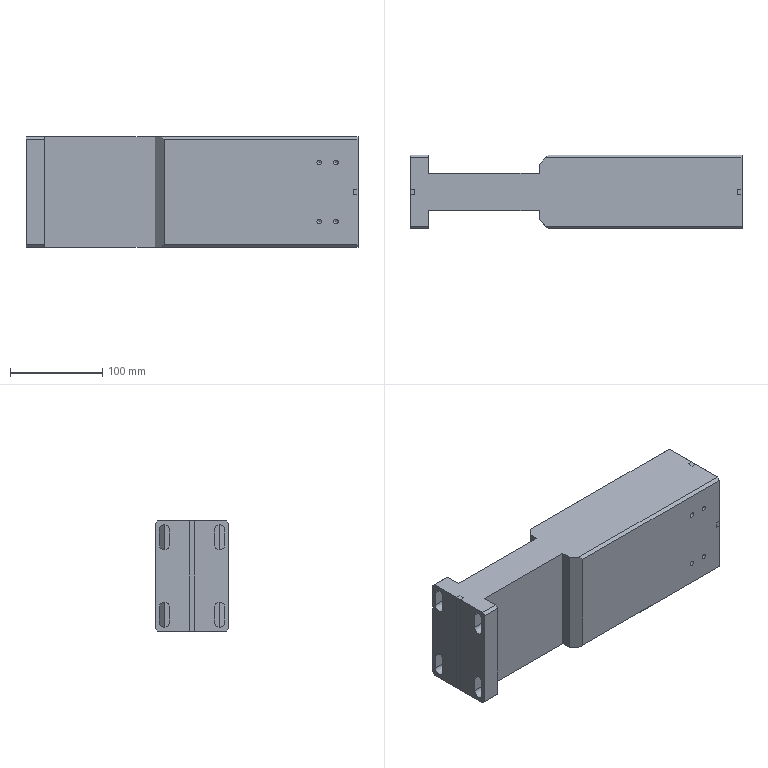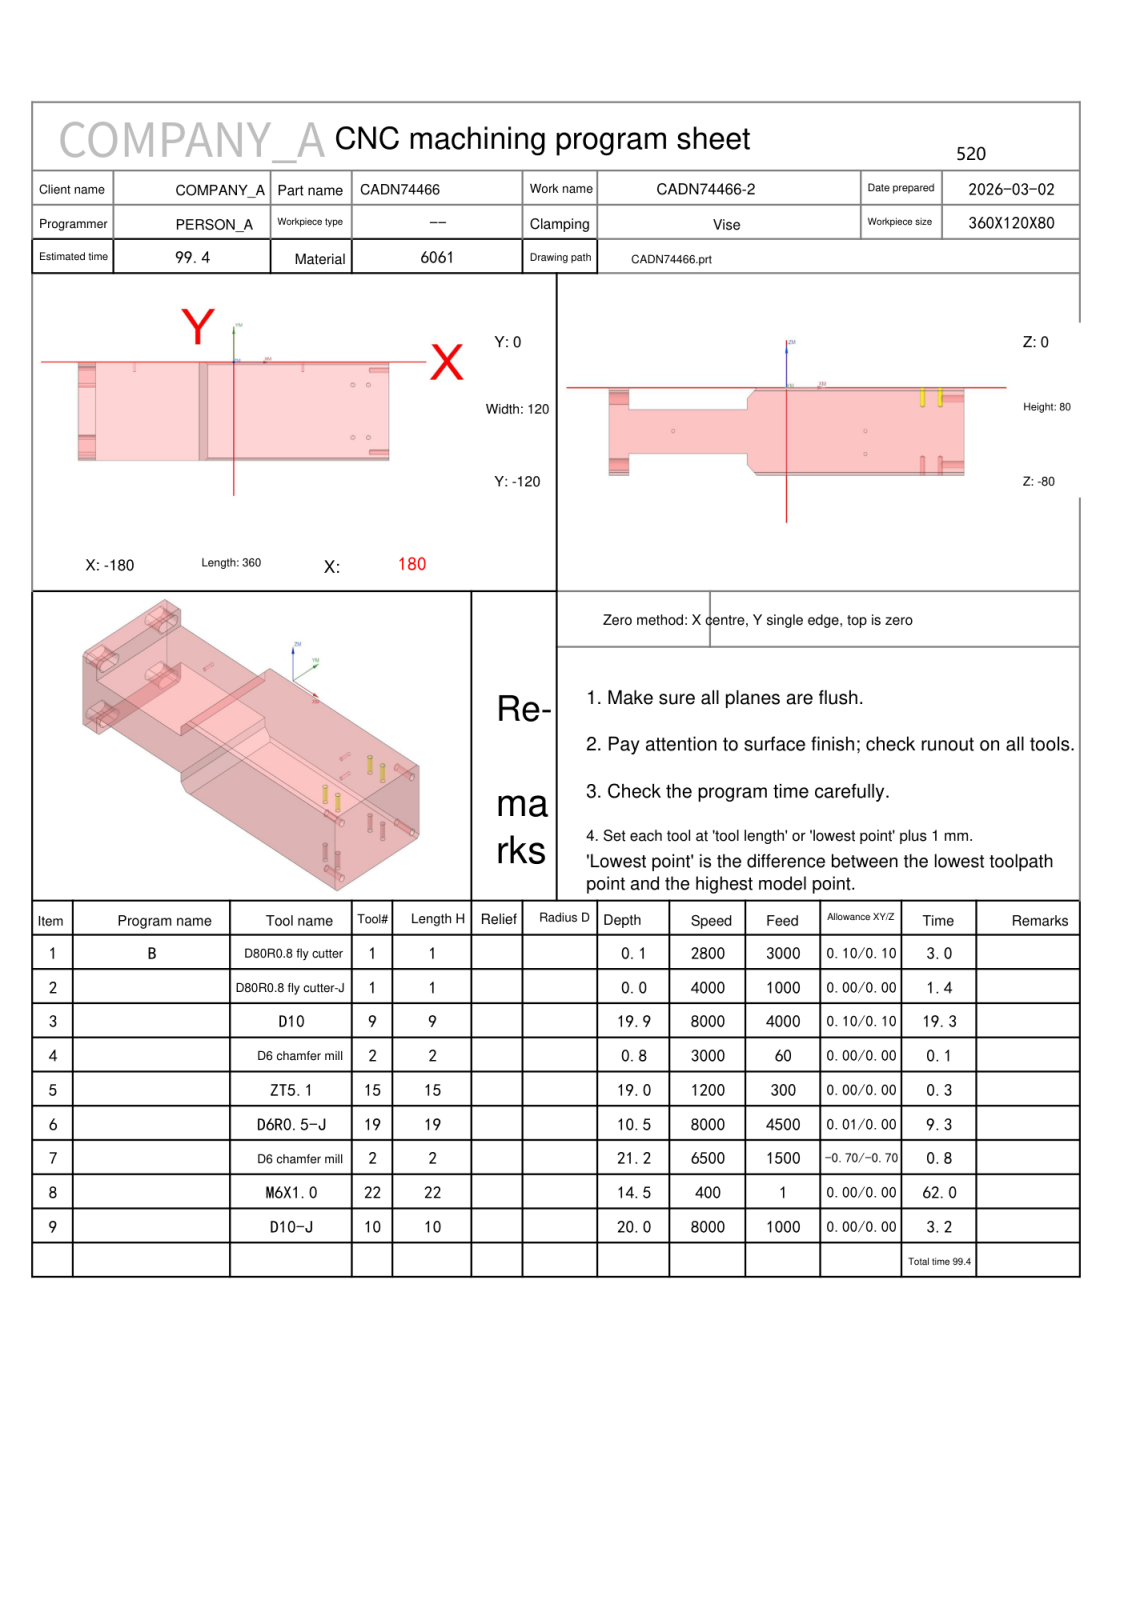NC program | NX | posted by the shop | part box 360 x 80 x 120 mm
Lines 1 to 150 of 6245:
%
O0001
(Machine time: 159.26 MIN)
(===Total Tool:7===)
(T1=D80R0.8 fly cutter D=80.  R=0.8  D-  H01 Z=0.    )
(T9=D10     D=10.  R=0.   D-  H09 Z=-19.9 )
(T2=D6 chamfer mill   D=6.   R=0.   D-  H02 Z=-21.2 )
(T15=ZT5.1  D=5.1  DR_a=118 D-  H15 Z=-19.  )
(T19=D6R0.5-J D=6.   R=0.5  D-  H19 Z=-10.5 )
(T22=M6X1.0 D=5.   DR_a=180 D-  H22 Z=-14.5 )
(T10=D10-J  D=10.  R=0.   D10 H10 Z=-20.  )
G80 G90 G17 G49 G40
G91 G28 Z0
M01
N1 T01 M06
(D80R0.8 fly cutter  D=80. R=0.8 H=01 ce=0.10 di=0.10)
G00 G90 G54 X232.097 Y-96.097 M03 S2800
G43 H01 Z50.
M08
Z6.011
G01 Z4.011 F3000.
X220.097
X-212.101
G02 X-220.097 Y-88.1 I.004 J8.
G01 Y-39.259
G02 X-212.101 Y-31.263 I8. J-.004
G01 X220.097
X232.097
Z6.011
G00 Y-96.097
Z5.522
G01 Z3.522
X220.097
X-212.101
G02 X-220.097 Y-88.1 I.004 J8.
G01 Y-39.259
G02 X-212.101 Y-31.263 I8. J-.004
G01 X220.097
X232.097
Z5.522
G00 Y-96.097
Z5.033
G01 Z3.033
X220.097
X-212.101
G02 X-220.097 Y-88.1 I.004 J8.
G01 Y-39.259
G02 X-212.101 Y-31.263 I8. J-.004
G01 X220.097
X232.097
Z5.033
G00 Y-96.097
Z4.544
G01 Z2.544
X220.097
X-212.101
G02 X-220.097 Y-88.1 I.004 J8.
G01 Y-39.259
G02 X-212.101 Y-31.263 I8. J-.004
G01 X220.097
X232.097
Z4.544
G00 Y-96.097
Z4.056
G01 Z2.056
X220.097
X-212.101
G02 X-220.097 Y-88.1 I.004 J8.
G01 Y-39.259
G02 X-212.101 Y-31.263 I8. J-.004
G01 X220.097
X232.097
Z4.056
G00 Y-96.097
Z3.567
G01 Z1.567
X220.097
X-212.101
G02 X-220.097 Y-88.1 I.004 J8.
G01 Y-39.259
G02 X-212.101 Y-31.263 I8. J-.004
G01 X220.097
X232.097
Z3.567
G00 Y-96.097
Z3.078
G01 Z1.078
X220.097
X-212.101
G02 X-220.097 Y-88.1 I.004 J8.
G01 Y-39.259
G02 X-212.101 Y-31.263 I8. J-.004
G01 X220.097
X232.097
Z3.078
G00 Y-96.097
Z2.589
G01 Z.589
X220.097
X-212.101
G02 X-220.097 Y-88.1 I.004 J8.
G01 Y-39.259
G02 X-212.101 Y-31.263 I8. J-.004
G01 X220.097
X232.097
Z2.589
G00 Y-96.097
Z2.1
G01 Z.1
X220.097
X-212.101
G02 X-220.097 Y-88.1 I.004 J8.
G01 Y-39.259
G02 X-212.101 Y-31.263 I8. J-.004
G01 X220.097
X232.097
Z2.1
G00 Z50.
G91 G28 Z0.0
M05
M09
G91 G28 Z0.0
M01
N2 T01 M06
(D80R0.8 fly cutter-J  D=80. R=0.8 H=01 ce=0.00 di=0.00)
G00 G90 G54 X231.999 Y-95.999 M03 S4000
G43 H01 Z50.
M08
Z2.
G01 Z0.0 F1000.
X219.999
X-212.799
G02 X-219.999 Y-88.799 I0.0 J7.2
G01 Y-71.68
G02 X-211.999 Y-63.68 I8. J0.0
G01 X212.799
G03 X219.999 Y-56.48 I0.0 J7.2
G01 Y-39.361
G03 X211.999 Y-31.361 I-8. J0.0
G01 X-219.999
X-231.999
Z2.
G00 Z50.
G91 G28 Z0.0
M05
M09
G91 G28 Z0.0
M01